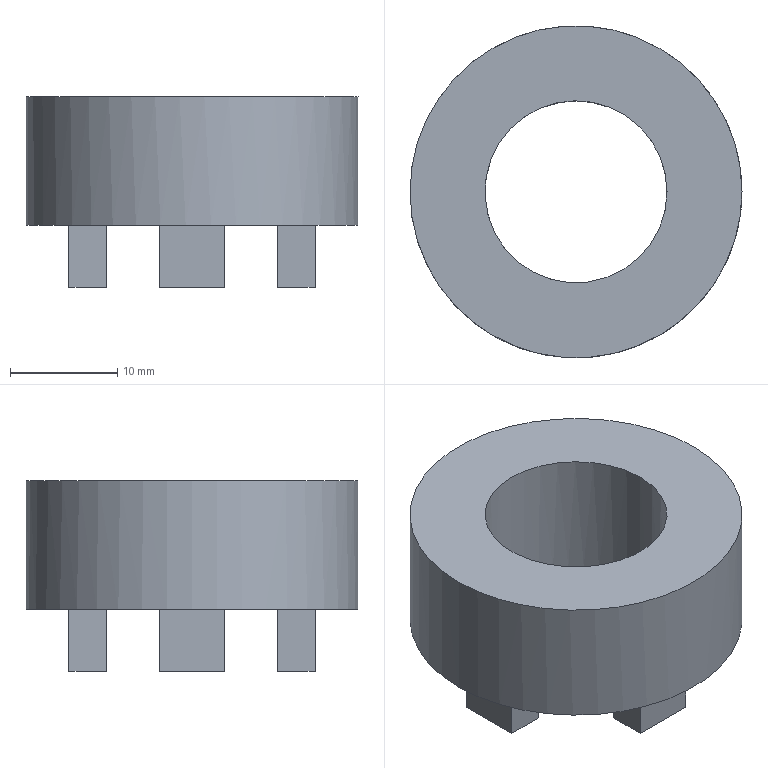Part | NX | features EXTRACT_BODY 3, EXTRUDE 3, DATUM_CSYS 1, LINKED_FACE 1, Pattern Geometry 1, REPLACE_FACE 1, SKETCH 1, UNITE 1 | 1 solid | 20 faces | box 31 x 31 x 17.802 mm | volume 6776 mm3 | plane 18 | cylinder 2 | commonest cylinder face diameters 17 x1 31 x1
STEP:
#1=CARTESIAN_POINT('',(-15.5,0.,-6.));
#2=VERTEX_POINT('',#1);
#3=CARTESIAN_POINT('',(0.,0.,-6.));
#4=DIRECTION('',(0.,0.,1.));
#5=DIRECTION('',(-1.,0.,0.));
#6=AXIS2_PLACEMENT_3D('',#3,#4,#5);
#7=CIRCLE('',#6,15.5);
#8=EDGE_CURVE('',#2,#2,#7,.T.);
#9=ORIENTED_EDGE('',*,*,#8,.F.);
#10=EDGE_LOOP('',(#9));
#11=FACE_BOUND('',#10,.T.);
#12=CARTESIAN_POINT('',(11.5,-3.,-6.));
#13=VERTEX_POINT('',#12);
#14=CARTESIAN_POINT('',(7.953,-3.,-6.));
#15=VERTEX_POINT('',#14);
#16=CARTESIAN_POINT('',(11.5,-3.,-6.));
#17=DIRECTION('',(-1.,0.,0.));
#18=VECTOR('',#17,1000.);
#19=LINE('',#16,#18);
#20=EDGE_CURVE('',#13,#15,#19,.T.);
#21=ORIENTED_EDGE('',*,*,#20,.F.);
#22=CARTESIAN_POINT('',(11.5,3.,-6.));
#23=VERTEX_POINT('',#22);
#24=CARTESIAN_POINT('',(11.5,3.,-6.));
#25=DIRECTION('',(0.,-1.,0.));
#26=VECTOR('',#25,1000.);
#27=LINE('',#24,#26);
#28=EDGE_CURVE('',#23,#13,#27,.T.);
#29=ORIENTED_EDGE('',*,*,#28,.F.);
#30=CARTESIAN_POINT('',(7.953,3.,-6.));
#31=VERTEX_POINT('',#30);
#32=CARTESIAN_POINT('',(7.953,3.,-6.));
#33=DIRECTION('',(1.,0.,0.));
#34=VECTOR('',#33,1000.);
#35=LINE('',#32,#34);
#36=EDGE_CURVE('',#31,#23,#35,.T.);
#37=ORIENTED_EDGE('',*,*,#36,.F.);
#38=CARTESIAN_POINT('',(3.,7.953,-6.));
#39=VERTEX_POINT('',#38);
#40=CARTESIAN_POINT('',(0.,0.,-6.));
#41=DIRECTION('',(0.,0.,1.));
#42=DIRECTION('',(1.,0.,0.));
#43=AXIS2_PLACEMENT_3D('',#40,#41,#42);
#44=CIRCLE('',#43,8.5);
#45=EDGE_CURVE('',#31,#39,#44,.T.);
#46=ORIENTED_EDGE('',*,*,#45,.T.);
#47=CARTESIAN_POINT('',(3.,11.5,-6.));
#48=VERTEX_POINT('',#47);
#49=CARTESIAN_POINT('',(3.,11.5,-6.));
#50=DIRECTION('',(0.,-1.,0.));
#51=VECTOR('',#50,1000.);
#52=LINE('',#49,#51);
#53=EDGE_CURVE('',#48,#39,#52,.T.);
#54=ORIENTED_EDGE('',*,*,#53,.F.);
#55=CARTESIAN_POINT('',(-3.,11.5,-6.));
#56=VERTEX_POINT('',#55);
#57=CARTESIAN_POINT('',(-3.,11.5,-6.));
#58=DIRECTION('',(1.,0.,0.));
#59=VECTOR('',#58,1000.);
#60=LINE('',#57,#59);
#61=EDGE_CURVE('',#56,#48,#60,.T.);
#62=ORIENTED_EDGE('',*,*,#61,.F.);
#63=CARTESIAN_POINT('',(-3.,7.953,-6.));
#64=VERTEX_POINT('',#63);
#65=CARTESIAN_POINT('',(-3.,7.953,-6.));
#66=DIRECTION('',(0.,1.,0.));
#67=VECTOR('',#66,1000.);
#68=LINE('',#65,#67);
#69=EDGE_CURVE('',#64,#56,#68,.T.);
#70=ORIENTED_EDGE('',*,*,#69,.F.);
#71=CARTESIAN_POINT('',(-7.953,3.,-6.));
#72=VERTEX_POINT('',#71);
#73=CARTESIAN_POINT('',(0.,0.,-6.));
#74=DIRECTION('',(0.,0.,1.));
#75=DIRECTION('',(1.,0.,0.));
#76=AXIS2_PLACEMENT_3D('',#73,#74,#75);
#77=CIRCLE('',#76,8.5);
#78=EDGE_CURVE('',#64,#72,#77,.T.);
#79=ORIENTED_EDGE('',*,*,#78,.T.);
#80=CARTESIAN_POINT('',(-11.5,3.,-6.));
#81=VERTEX_POINT('',#80);
#82=CARTESIAN_POINT('',(0.,3.,-6.));
#83=DIRECTION('',(-1.,0.,0.));
#84=VECTOR('',#83,1000.);
#85=LINE('',#82,#84);
#86=EDGE_CURVE('',#72,#81,#85,.T.);
#87=ORIENTED_EDGE('',*,*,#86,.T.);
#88=CARTESIAN_POINT('',(-11.5,-3.,-6.));
#89=VERTEX_POINT('',#88);
#90=CARTESIAN_POINT('',(-11.5,0.,-6.));
#91=DIRECTION('',(0.,-1.,0.));
#92=VECTOR('',#91,1000.);
#93=LINE('',#90,#92);
#94=EDGE_CURVE('',#81,#89,#93,.T.);
#95=ORIENTED_EDGE('',*,*,#94,.T.);
#96=CARTESIAN_POINT('',(-7.953,-3.,-6.));
#97=VERTEX_POINT('',#96);
#98=CARTESIAN_POINT('',(0.,-3.,-6.));
#99=DIRECTION('',(1.,0.,0.));
#100=VECTOR('',#99,1000.);
#101=LINE('',#98,#100);
#102=EDGE_CURVE('',#89,#97,#101,.T.);
#103=ORIENTED_EDGE('',*,*,#102,.T.);
#104=CARTESIAN_POINT('',(-3.,-7.953,-6.));
#105=VERTEX_POINT('',#104);
#106=CARTESIAN_POINT('',(0.,0.,-6.));
#107=DIRECTION('',(0.,0.,1.));
#108=DIRECTION('',(1.,0.,0.));
#109=AXIS2_PLACEMENT_3D('',#106,#107,#108);
#110=CIRCLE('',#109,8.5);
#111=EDGE_CURVE('',#97,#105,#110,.T.);
#112=ORIENTED_EDGE('',*,*,#111,.T.);
#113=CARTESIAN_POINT('',(-3.,-11.5,-6.));
#114=VERTEX_POINT('',#113);
#115=CARTESIAN_POINT('',(-3.,-11.5,-6.));
#116=DIRECTION('',(0.,1.,0.));
#117=VECTOR('',#116,1000.);
#118=LINE('',#115,#117);
#119=EDGE_CURVE('',#114,#105,#118,.T.);
#120=ORIENTED_EDGE('',*,*,#119,.F.);
#121=CARTESIAN_POINT('',(3.,-11.5,-6.));
#122=VERTEX_POINT('',#121);
#123=CARTESIAN_POINT('',(3.,-11.5,-6.));
#124=DIRECTION('',(-1.,0.,0.));
#125=VECTOR('',#124,1000.);
#126=LINE('',#123,#125);
#127=EDGE_CURVE('',#122,#114,#126,.T.);
#128=ORIENTED_EDGE('',*,*,#127,.F.);
#129=CARTESIAN_POINT('',(3.,-7.953,-6.));
#130=VERTEX_POINT('',#129);
#131=CARTESIAN_POINT('',(3.,-7.953,-6.));
#132=DIRECTION('',(0.,-1.,0.));
#133=VECTOR('',#132,1000.);
#134=LINE('',#131,#133);
#135=EDGE_CURVE('',#130,#122,#134,.T.);
#136=ORIENTED_EDGE('',*,*,#135,.F.);
#137=CARTESIAN_POINT('',(0.,0.,-6.));
#138=DIRECTION('',(0.,0.,1.));
#139=DIRECTION('',(1.,0.,0.));
#140=AXIS2_PLACEMENT_3D('',#137,#138,#139);
#141=CIRCLE('',#140,8.5);
#142=EDGE_CURVE('',#130,#15,#141,.T.);
#143=ORIENTED_EDGE('',*,*,#142,.T.);
#144=EDGE_LOOP('',(#21,#29,#37,#46,#54,#62,#70,#79,#87,#95,#103,#112,#120,#128,#136,#143));
#145=FACE_BOUND('',#144,.T.);
#146=CARTESIAN_POINT('',(0.,0.,-6.));
#147=DIRECTION('',(0.,0.,1.));
#148=DIRECTION('',(1.,0.,0.));
#149=AXIS2_PLACEMENT_3D('',#146,#147,#148);
#150=PLANE('',#149);
#151=ADVANCED_FACE('',(#11,#145),#150,.F.);
#152=ORIENTED_EDGE('',*,*,#8,.T.);
#153=EDGE_LOOP('',(#152));
#154=FACE_BOUND('',#153,.T.);
#155=CARTESIAN_POINT('',(15.5,0.,6.));
#156=VERTEX_POINT('',#155);
#157=CARTESIAN_POINT('',(0.,0.,6.));
#158=DIRECTION('',(0.,0.,1.));
#159=DIRECTION('',(1.,0.,0.));
#160=AXIS2_PLACEMENT_3D('',#157,#158,#159);
#161=CIRCLE('',#160,15.5);
#162=EDGE_CURVE('',#156,#156,#161,.T.);
#163=ORIENTED_EDGE('',*,*,#162,.F.);
#164=EDGE_LOOP('',(#163));
#165=FACE_BOUND('',#164,.T.);
#166=CARTESIAN_POINT('',(0.,0.,6.));
#167=DIRECTION('',(0.,0.,-1.));
#168=DIRECTION('',(-1.,0.,0.));
#169=AXIS2_PLACEMENT_3D('',#166,#167,#168);
#170=CYLINDRICAL_SURFACE('',#169,15.5);
#171=ADVANCED_FACE('',(#154,#165),#170,.T.);
#172=CARTESIAN_POINT('',(8.5,0.,6.));
#173=VERTEX_POINT('',#172);
#174=CARTESIAN_POINT('',(0.,0.,6.));
#175=DIRECTION('',(0.,0.,1.));
#176=DIRECTION('',(1.,0.,0.));
#177=AXIS2_PLACEMENT_3D('',#174,#175,#176);
#178=CIRCLE('',#177,8.5);
#179=EDGE_CURVE('',#173,#173,#178,.T.);
#180=ORIENTED_EDGE('',*,*,#179,.F.);
#181=EDGE_LOOP('',(#180));
#182=FACE_BOUND('',#181,.T.);
#183=ORIENTED_EDGE('',*,*,#162,.T.);
#184=EDGE_LOOP('',(#183));
#185=FACE_BOUND('',#184,.T.);
#186=CARTESIAN_POINT('',(0.,0.,6.));
#187=DIRECTION('',(0.,0.,1.));
#188=DIRECTION('',(1.,0.,0.));
#189=AXIS2_PLACEMENT_3D('',#186,#187,#188);
#190=PLANE('',#189);
#191=ADVANCED_FACE('',(#182,#185),#190,.T.);
#192=ORIENTED_EDGE('',*,*,#179,.T.);
#193=EDGE_LOOP('',(#192));
#194=FACE_BOUND('',#193,.T.);
#195=ORIENTED_EDGE('',*,*,#111,.F.);
#196=CARTESIAN_POINT('',(-7.953,-3.,-11.802));
#197=VERTEX_POINT('',#196);
#198=CARTESIAN_POINT('',(-7.953,-3.,-6.));
#199=DIRECTION('',(0.,0.,-1.));
#200=VECTOR('',#199,1000.);
#201=LINE('',#198,#200);
#202=EDGE_CURVE('',#97,#197,#201,.T.);
#203=ORIENTED_EDGE('',*,*,#202,.T.);
#204=CARTESIAN_POINT('',(-7.953,3.,-11.802));
#205=VERTEX_POINT('',#204);
#206=CARTESIAN_POINT('',(0.,0.,-11.802));
#207=DIRECTION('',(0.,0.,1.));
#208=DIRECTION('',(-0.9356,0.3529,0.));
#209=AXIS2_PLACEMENT_3D('',#206,#207,#208);
#210=CIRCLE('',#209,8.5);
#211=EDGE_CURVE('',#205,#197,#210,.T.);
#212=ORIENTED_EDGE('',*,*,#211,.F.);
#213=CARTESIAN_POINT('',(-7.953,3.,-6.));
#214=DIRECTION('',(0.,0.,-1.));
#215=VECTOR('',#214,1000.);
#216=LINE('',#213,#215);
#217=EDGE_CURVE('',#72,#205,#216,.T.);
#218=ORIENTED_EDGE('',*,*,#217,.F.);
#219=ORIENTED_EDGE('',*,*,#78,.F.);
#220=CARTESIAN_POINT('',(-3.,7.953,-11.802));
#221=VERTEX_POINT('',#220);
#222=CARTESIAN_POINT('',(-3.,7.953,-6.));
#223=DIRECTION('',(0.,0.,-1.));
#224=VECTOR('',#223,1000.);
#225=LINE('',#222,#224);
#226=EDGE_CURVE('',#64,#221,#225,.T.);
#227=ORIENTED_EDGE('',*,*,#226,.T.);
#228=CARTESIAN_POINT('',(3.,7.953,-11.802));
#229=VERTEX_POINT('',#228);
#230=CARTESIAN_POINT('',(0.,0.,-11.802));
#231=DIRECTION('',(0.,0.,1.));
#232=DIRECTION('',(0.3529,0.9356,0.));
#233=AXIS2_PLACEMENT_3D('',#230,#231,#232);
#234=CIRCLE('',#233,8.5);
#235=EDGE_CURVE('',#229,#221,#234,.T.);
#236=ORIENTED_EDGE('',*,*,#235,.F.);
#237=CARTESIAN_POINT('',(3.,7.953,-6.));
#238=DIRECTION('',(0.,0.,-1.));
#239=VECTOR('',#238,1000.);
#240=LINE('',#237,#239);
#241=EDGE_CURVE('',#39,#229,#240,.T.);
#242=ORIENTED_EDGE('',*,*,#241,.F.);
#243=ORIENTED_EDGE('',*,*,#45,.F.);
#244=CARTESIAN_POINT('',(7.953,3.,-11.802));
#245=VERTEX_POINT('',#244);
#246=CARTESIAN_POINT('',(7.953,3.,-6.));
#247=DIRECTION('',(0.,0.,-1.));
#248=VECTOR('',#247,1000.);
#249=LINE('',#246,#248);
#250=EDGE_CURVE('',#31,#245,#249,.T.);
#251=ORIENTED_EDGE('',*,*,#250,.T.);
#252=CARTESIAN_POINT('',(7.953,-3.,-11.802));
#253=VERTEX_POINT('',#252);
#254=CARTESIAN_POINT('',(0.,0.,-11.802));
#255=DIRECTION('',(0.,0.,1.));
#256=DIRECTION('',(0.9356,-0.3529,0.));
#257=AXIS2_PLACEMENT_3D('',#254,#255,#256);
#258=CIRCLE('',#257,8.5);
#259=EDGE_CURVE('',#253,#245,#258,.T.);
#260=ORIENTED_EDGE('',*,*,#259,.F.);
#261=CARTESIAN_POINT('',(7.953,-3.,-6.));
#262=DIRECTION('',(0.,0.,-1.));
#263=VECTOR('',#262,1000.);
#264=LINE('',#261,#263);
#265=EDGE_CURVE('',#15,#253,#264,.T.);
#266=ORIENTED_EDGE('',*,*,#265,.F.);
#267=ORIENTED_EDGE('',*,*,#142,.F.);
#268=CARTESIAN_POINT('',(3.,-7.953,-11.802));
#269=VERTEX_POINT('',#268);
#270=CARTESIAN_POINT('',(3.,-7.953,-6.));
#271=DIRECTION('',(0.,0.,-1.));
#272=VECTOR('',#271,1000.);
#273=LINE('',#270,#272);
#274=EDGE_CURVE('',#130,#269,#273,.T.);
#275=ORIENTED_EDGE('',*,*,#274,.T.);
#276=CARTESIAN_POINT('',(-3.,-7.953,-11.802));
#277=VERTEX_POINT('',#276);
#278=CARTESIAN_POINT('',(0.,0.,-11.802));
#279=DIRECTION('',(0.,0.,1.));
#280=DIRECTION('',(-0.3529,-0.9356,0.));
#281=AXIS2_PLACEMENT_3D('',#278,#279,#280);
#282=CIRCLE('',#281,8.5);
#283=EDGE_CURVE('',#277,#269,#282,.T.);
#284=ORIENTED_EDGE('',*,*,#283,.F.);
#285=CARTESIAN_POINT('',(-3.,-7.953,-6.));
#286=DIRECTION('',(0.,0.,-1.));
#287=VECTOR('',#286,1000.);
#288=LINE('',#285,#287);
#289=EDGE_CURVE('',#105,#277,#288,.T.);
#290=ORIENTED_EDGE('',*,*,#289,.F.);
#291=EDGE_LOOP('',(#195,#203,#212,#218,#219,#227,#236,#242,#243,#251,#260,#266,#267,#275,#284,#290));
#292=FACE_BOUND('',#291,.T.);
#293=CARTESIAN_POINT('',(0.,0.,18.198));
#294=DIRECTION('',(0.,0.,-1.));
#295=DIRECTION('',(-1.,0.,0.));
#296=AXIS2_PLACEMENT_3D('',#293,#294,#295);
#297=CYLINDRICAL_SURFACE('',#296,8.5);
#298=ADVANCED_FACE('',(#194,#292),#297,.F.);
#299=CARTESIAN_POINT('',(-3.,-11.5,-11.802));
#300=VERTEX_POINT('',#299);
#301=CARTESIAN_POINT('',(-3.,-11.5,-11.802));
#302=DIRECTION('',(0.,1.,0.));
#303=VECTOR('',#302,1000.);
#304=LINE('',#301,#303);
#305=EDGE_CURVE('',#300,#277,#304,.T.);
#306=ORIENTED_EDGE('',*,*,#305,.F.);
#307=CARTESIAN_POINT('',(-3.,-11.5,-6.));
#308=DIRECTION('',(0.,0.,-1.));
#309=VECTOR('',#308,1000.);
#310=LINE('',#307,#309);
#311=EDGE_CURVE('',#114,#300,#310,.T.);
#312=ORIENTED_EDGE('',*,*,#311,.F.);
#313=ORIENTED_EDGE('',*,*,#119,.T.);
#314=ORIENTED_EDGE('',*,*,#289,.T.);
#315=EDGE_LOOP('',(#306,#312,#313,#314));
#316=FACE_BOUND('',#315,.T.);
#317=CARTESIAN_POINT('',(-3.,-11.5,-6.));
#318=DIRECTION('',(-1.,0.,0.));
#319=DIRECTION('',(0.,0.,1.));
#320=AXIS2_PLACEMENT_3D('',#317,#318,#319);
#321=PLANE('',#320);
#322=ADVANCED_FACE('',(#316),#321,.T.);
#323=CARTESIAN_POINT('',(3.,-11.5,-11.802));
#324=VERTEX_POINT('',#323);
#325=CARTESIAN_POINT('',(3.,-7.953,-11.802));
#326=DIRECTION('',(0.,-1.,0.));
#327=VECTOR('',#326,1000.);
#328=LINE('',#325,#327);
#329=EDGE_CURVE('',#269,#324,#328,.T.);
#330=ORIENTED_EDGE('',*,*,#329,.F.);
#331=ORIENTED_EDGE('',*,*,#274,.F.);
#332=ORIENTED_EDGE('',*,*,#135,.T.);
#333=CARTESIAN_POINT('',(3.,-11.5,-6.));
#334=DIRECTION('',(0.,0.,-1.));
#335=VECTOR('',#334,1000.);
#336=LINE('',#333,#335);
#337=EDGE_CURVE('',#122,#324,#336,.T.);
#338=ORIENTED_EDGE('',*,*,#337,.T.);
#339=EDGE_LOOP('',(#330,#331,#332,#338));
#340=FACE_BOUND('',#339,.T.);
#341=CARTESIAN_POINT('',(3.,-7.953,-6.));
#342=DIRECTION('',(1.,0.,0.));
#343=DIRECTION('',(0.,0.,-1.));
#344=AXIS2_PLACEMENT_3D('',#341,#342,#343);
#345=PLANE('',#344);
#346=ADVANCED_FACE('',(#340),#345,.T.);
#347=CARTESIAN_POINT('',(3.,-11.5,-11.802));
#348=DIRECTION('',(-1.,0.,0.));
#349=VECTOR('',#348,1000.);
#350=LINE('',#347,#349);
#351=EDGE_CURVE('',#324,#300,#350,.T.);
#352=ORIENTED_EDGE('',*,*,#351,.F.);
#353=ORIENTED_EDGE('',*,*,#337,.F.);
#354=ORIENTED_EDGE('',*,*,#127,.T.);
#355=ORIENTED_EDGE('',*,*,#311,.T.);
#356=EDGE_LOOP('',(#352,#353,#354,#355));
#357=FACE_BOUND('',#356,.T.);
#358=CARTESIAN_POINT('',(3.,-11.5,-6.));
#359=DIRECTION('',(0.,-1.,0.));
#360=DIRECTION('',(0.,0.,-1.));
#361=AXIS2_PLACEMENT_3D('',#358,#359,#360);
#362=PLANE('',#361);
#363=ADVANCED_FACE('',(#357),#362,.T.);
#364=ORIENTED_EDGE('',*,*,#305,.T.);
#365=ORIENTED_EDGE('',*,*,#283,.T.);
#366=ORIENTED_EDGE('',*,*,#329,.T.);
#367=ORIENTED_EDGE('',*,*,#351,.T.);
#368=EDGE_LOOP('',(#364,#365,#366,#367));
#369=FACE_BOUND('',#368,.T.);
#370=CARTESIAN_POINT('',(0.,0.,-11.802));
#371=DIRECTION('',(0.,0.,1.));
#372=DIRECTION('',(1.,0.,0.));
#373=AXIS2_PLACEMENT_3D('',#370,#371,#372);
#374=PLANE('',#373);
#375=ADVANCED_FACE('',(#369),#374,.F.);
#376=ORIENTED_EDGE('',*,*,#94,.F.);
#377=CARTESIAN_POINT('',(-11.5,3.,-11.802));
#378=VERTEX_POINT('',#377);
#379=CARTESIAN_POINT('',(-11.5,3.,-6.));
#380=DIRECTION('',(0.,0.,-1.));
#381=VECTOR('',#380,1000.);
#382=LINE('',#379,#381);
#383=EDGE_CURVE('',#81,#378,#382,.T.);
#384=ORIENTED_EDGE('',*,*,#383,.T.);
#385=CARTESIAN_POINT('',(-11.5,-3.,-11.802));
#386=VERTEX_POINT('',#385);
#387=CARTESIAN_POINT('',(-11.5,-3.,-11.802));
#388=DIRECTION('',(0.,1.,0.));
#389=VECTOR('',#388,1000.);
#390=LINE('',#387,#389);
#391=EDGE_CURVE('',#386,#378,#390,.T.);
#392=ORIENTED_EDGE('',*,*,#391,.F.);
#393=CARTESIAN_POINT('',(-11.5,-3.,-6.));
#394=DIRECTION('',(0.,0.,-1.));
#395=VECTOR('',#394,1000.);
#396=LINE('',#393,#395);
#397=EDGE_CURVE('',#89,#386,#396,.T.);
#398=ORIENTED_EDGE('',*,*,#397,.F.);
#399=EDGE_LOOP('',(#376,#384,#392,#398));
#400=FACE_BOUND('',#399,.T.);
#401=CARTESIAN_POINT('',(-11.5,-3.,-6.));
#402=DIRECTION('',(-1.,0.,0.));
#403=DIRECTION('',(0.,0.,-1.));
#404=AXIS2_PLACEMENT_3D('',#401,#402,#403);
#405=PLANE('',#404);
#406=ADVANCED_FACE('',(#400),#405,.T.);
#407=ORIENTED_EDGE('',*,*,#86,.F.);
#408=ORIENTED_EDGE('',*,*,#217,.T.);
#409=CARTESIAN_POINT('',(-11.5,3.,-11.802));
#410=DIRECTION('',(1.,0.,0.));
#411=VECTOR('',#410,1000.);
#412=LINE('',#409,#411);
#413=EDGE_CURVE('',#378,#205,#412,.T.);
#414=ORIENTED_EDGE('',*,*,#413,.F.);
#415=ORIENTED_EDGE('',*,*,#383,.F.);
#416=EDGE_LOOP('',(#407,#408,#414,#415));
#417=FACE_BOUND('',#416,.T.);
#418=CARTESIAN_POINT('',(-11.5,3.,-6.));
#419=DIRECTION('',(0.,1.,0.));
#420=DIRECTION('',(0.,0.,1.));
#421=AXIS2_PLACEMENT_3D('',#418,#419,#420);
#422=PLANE('',#421);
#423=ADVANCED_FACE('',(#417),#422,.T.);
#424=ORIENTED_EDGE('',*,*,#102,.F.);
#425=ORIENTED_EDGE('',*,*,#397,.T.);
#426=CARTESIAN_POINT('',(-7.953,-3.,-11.802));
#427=DIRECTION('',(-1.,0.,0.));
#428=VECTOR('',#427,1000.);
#429=LINE('',#426,#428);
#430=EDGE_CURVE('',#197,#386,#429,.T.);
#431=ORIENTED_EDGE('',*,*,#430,.F.);
#432=ORIENTED_EDGE('',*,*,#202,.F.);
#433=EDGE_LOOP('',(#424,#425,#431,#432));
#434=FACE_BOUND('',#433,.T.);
#435=CARTESIAN_POINT('',(-7.953,-3.,-6.));
#436=DIRECTION('',(0.,-1.,0.));
#437=DIRECTION('',(0.,0.,-1.));
#438=AXIS2_PLACEMENT_3D('',#435,#436,#437);
#439=PLANE('',#438);
#440=ADVANCED_FACE('',(#434),#439,.T.);
#441=ORIENTED_EDGE('',*,*,#413,.T.);
#442=ORIENTED_EDGE('',*,*,#211,.T.);
#443=ORIENTED_EDGE('',*,*,#430,.T.);
#444=ORIENTED_EDGE('',*,*,#391,.T.);
#445=EDGE_LOOP('',(#441,#442,#443,#444));
#446=FACE_BOUND('',#445,.T.);
#447=CARTESIAN_POINT('',(0.,0.,-11.802));
#448=DIRECTION('',(0.,0.,1.));
#449=DIRECTION('',(0.,-1.,0.));
#450=AXIS2_PLACEMENT_3D('',#447,#448,#449);
#451=PLANE('',#450);
#452=ADVANCED_FACE('',(#446),#451,.F.);
#453=CARTESIAN_POINT('',(3.,11.5,-11.802));
#454=VERTEX_POINT('',#453);
#455=CARTESIAN_POINT('',(3.,11.5,-11.802));
#456=DIRECTION('',(0.,-1.,0.));
#457=VECTOR('',#456,1000.);
#458=LINE('',#455,#457);
#459=EDGE_CURVE('',#454,#229,#458,.T.);
#460=ORIENTED_EDGE('',*,*,#459,.F.);
#461=CARTESIAN_POINT('',(3.,11.5,-6.));
#462=DIRECTION('',(0.,0.,-1.));
#463=VECTOR('',#462,1000.);
#464=LINE('',#461,#463);
#465=EDGE_CURVE('',#48,#454,#464,.T.);
#466=ORIENTED_EDGE('',*,*,#465,.F.);
#467=ORIENTED_EDGE('',*,*,#53,.T.);
#468=ORIENTED_EDGE('',*,*,#241,.T.);
#469=EDGE_LOOP('',(#460,#466,#467,#468));
#470=FACE_BOUND('',#469,.T.);
#471=CARTESIAN_POINT('',(3.,11.5,-6.));
#472=DIRECTION('',(1.,0.,0.));
#473=DIRECTION('',(0.,0.,1.));
#474=AXIS2_PLACEMENT_3D('',#471,#472,#473);
#475=PLANE('',#474);
#476=ADVANCED_FACE('',(#470),#475,.T.);
#477=CARTESIAN_POINT('',(-3.,11.5,-11.802));
#478=VERTEX_POINT('',#477);
#479=CARTESIAN_POINT('',(-3.,7.953,-11.802));
#480=DIRECTION('',(0.,1.,0.));
#481=VECTOR('',#480,1000.);
#482=LINE('',#479,#481);
#483=EDGE_CURVE('',#221,#478,#482,.T.);
#484=ORIENTED_EDGE('',*,*,#483,.F.);
#485=ORIENTED_EDGE('',*,*,#226,.F.);
#486=ORIENTED_EDGE('',*,*,#69,.T.);
#487=CARTESIAN_POINT('',(-3.,11.5,-6.));
#488=DIRECTION('',(0.,0.,-1.));
#489=VECTOR('',#488,1000.);
#490=LINE('',#487,#489);
#491=EDGE_CURVE('',#56,#478,#490,.T.);
#492=ORIENTED_EDGE('',*,*,#491,.T.);
#493=EDGE_LOOP('',(#484,#485,#486,#492));
#494=FACE_BOUND('',#493,.T.);
#495=CARTESIAN_POINT('',(-3.,7.953,-6.));
#496=DIRECTION('',(-1.,0.,0.));
#497=DIRECTION('',(0.,0.,-1.));
#498=AXIS2_PLACEMENT_3D('',#495,#496,#497);
#499=PLANE('',#498);
#500=ADVANCED_FACE('',(#494),#499,.T.);
#501=CARTESIAN_POINT('',(-3.,11.5,-11.802));
#502=DIRECTION('',(1.,0.,0.));
#503=VECTOR('',#502,1000.);
#504=LINE('',#501,#503);
#505=EDGE_CURVE('',#478,#454,#504,.T.);
#506=ORIENTED_EDGE('',*,*,#505,.F.);
#507=ORIENTED_EDGE('',*,*,#491,.F.);
#508=ORIENTED_EDGE('',*,*,#61,.T.);
#509=ORIENTED_EDGE('',*,*,#465,.T.);
#510=EDGE_LOOP('',(#506,#507,#508,#509));
#511=FACE_BOUND('',#510,.T.);
#512=CARTESIAN_POINT('',(-3.,11.5,-6.));
#513=DIRECTION('',(0.,1.,0.));
#514=DIRECTION('',(0.,0.,-1.));
#515=AXIS2_PLACEMENT_3D('',#512,#513,#514);
#516=PLANE('',#515);
#517=ADVANCED_FACE('',(#511),#516,.T.);
#518=ORIENTED_EDGE('',*,*,#459,.T.);
#519=ORIENTED_EDGE('',*,*,#235,.T.);
#520=ORIENTED_EDGE('',*,*,#483,.T.);
#521=ORIENTED_EDGE('',*,*,#505,.T.);
#522=EDGE_LOOP('',(#518,#519,#520,#521));
#523=FACE_BOUND('',#522,.T.);
#524=CARTESIAN_POINT('',(0.,0.,-11.802));
#525=DIRECTION('',(0.,0.,1.));
#526=DIRECTION('',(-1.,0.,0.));
#527=AXIS2_PLACEMENT_3D('',#524,#525,#526);
#528=PLANE('',#527);
#529=ADVANCED_FACE('',(#523),#528,.F.);
#530=CARTESIAN_POINT('',(11.5,-3.,-11.802));
#531=VERTEX_POINT('',#530);
#532=CARTESIAN_POINT('',(11.5,-3.,-11.802));
#533=DIRECTION('',(-1.,0.,0.));
#534=VECTOR('',#533,1000.);
#535=LINE('',#532,#534);
#536=EDGE_CURVE('',#531,#253,#535,.T.);
#537=ORIENTED_EDGE('',*,*,#536,.F.);
#538=CARTESIAN_POINT('',(11.5,-3.,-6.));
#539=DIRECTION('',(0.,0.,-1.));
#540=VECTOR('',#539,1000.);
#541=LINE('',#538,#540);
#542=EDGE_CURVE('',#13,#531,#541,.T.);
#543=ORIENTED_EDGE('',*,*,#542,.F.);
#544=ORIENTED_EDGE('',*,*,#20,.T.);
#545=ORIENTED_EDGE('',*,*,#265,.T.);
#546=EDGE_LOOP('',(#537,#543,#544,#545));
#547=FACE_BOUND('',#546,.T.);
#548=CARTESIAN_POINT('',(11.5,-3.,-6.));
#549=DIRECTION('',(0.,-1.,0.));
#550=DIRECTION('',(0.,0.,1.));
#551=AXIS2_PLACEMENT_3D('',#548,#549,#550);
#552=PLANE('',#551);
#553=ADVANCED_FACE('',(#547),#552,.T.);
#554=CARTESIAN_POINT('',(11.5,3.,-11.802));
#555=VERTEX_POINT('',#554);
#556=CARTESIAN_POINT('',(7.953,3.,-11.802));
#557=DIRECTION('',(1.,0.,0.));
#558=VECTOR('',#557,1000.);
#559=LINE('',#556,#558);
#560=EDGE_CURVE('',#245,#555,#559,.T.);
#561=ORIENTED_EDGE('',*,*,#560,.F.);
#562=ORIENTED_EDGE('',*,*,#250,.F.);
#563=ORIENTED_EDGE('',*,*,#36,.T.);
#564=CARTESIAN_POINT('',(11.5,3.,-6.));
#565=DIRECTION('',(0.,0.,-1.));
#566=VECTOR('',#565,1000.);
#567=LINE('',#564,#566);
#568=EDGE_CURVE('',#23,#555,#567,.T.);
#569=ORIENTED_EDGE('',*,*,#568,.T.);
#570=EDGE_LOOP('',(#561,#562,#563,#569));
#571=FACE_BOUND('',#570,.T.);
#572=CARTESIAN_POINT('',(7.953,3.,-6.));
#573=DIRECTION('',(0.,1.,0.));
#574=DIRECTION('',(0.,0.,-1.));
#575=AXIS2_PLACEMENT_3D('',#572,#573,#574);
#576=PLANE('',#575);
#577=ADVANCED_FACE('',(#571),#576,.T.);
#578=CARTESIAN_POINT('',(11.5,3.,-11.802));
#579=DIRECTION('',(0.,-1.,0.));
#580=VECTOR('',#579,1000.);
#581=LINE('',#578,#580);
#582=EDGE_CURVE('',#555,#531,#581,.T.);
#583=ORIENTED_EDGE('',*,*,#582,.F.);
#584=ORIENTED_EDGE('',*,*,#568,.F.);
#585=ORIENTED_EDGE('',*,*,#28,.T.);
#586=ORIENTED_EDGE('',*,*,#542,.T.);
#587=EDGE_LOOP('',(#583,#584,#585,#586));
#588=FACE_BOUND('',#587,.T.);
#589=CARTESIAN_POINT('',(11.5,3.,-6.));
#590=DIRECTION('',(1.,0.,0.));
#591=DIRECTION('',(0.,0.,-1.));
#592=AXIS2_PLACEMENT_3D('',#589,#590,#591);
#593=PLANE('',#592);
#594=ADVANCED_FACE('',(#588),#593,.T.);
#595=ORIENTED_EDGE('',*,*,#536,.T.);
#596=ORIENTED_EDGE('',*,*,#259,.T.);
#597=ORIENTED_EDGE('',*,*,#560,.T.);
#598=ORIENTED_EDGE('',*,*,#582,.T.);
#599=EDGE_LOOP('',(#595,#596,#597,#598));
#600=FACE_BOUND('',#599,.T.);
#601=CARTESIAN_POINT('',(0.,0.,-11.802));
#602=DIRECTION('',(0.,0.,1.));
#603=DIRECTION('',(0.,1.,0.));
#604=AXIS2_PLACEMENT_3D('',#601,#602,#603);
#605=PLANE('',#604);
#606=ADVANCED_FACE('',(#600),#605,.F.);
#607=CLOSED_SHELL('',(#151,#171,#191,#298,#322,#346,#363,#375,#406,#423,#440,#452,#476,#500,#517,#529,#553,#577,#594,#606));
#608=MANIFOLD_SOLID_BREP('',#607);
#609=(LENGTH_UNIT()NAMED_UNIT(*)SI_UNIT(.MILLI.,.METRE.));
#610=UNCERTAINTY_MEASURE_WITH_UNIT(LENGTH_MEASURE(0.00001),#609,'','');
#611=(NAMED_UNIT(*)PLANE_ANGLE_UNIT()SI_UNIT($,.RADIAN.));
#612=(NAMED_UNIT(*)SI_UNIT($,.STERADIAN.)SOLID_ANGLE_UNIT());
#613=(GEOMETRIC_REPRESENTATION_CONTEXT(3)GLOBAL_UNCERTAINTY_ASSIGNED_CONTEXT((#610))GLOBAL_UNIT_ASSIGNED_CONTEXT((#609,#611,#612))REPRESENTATION_CONTEXT('',''));
#614=ADVANCED_BREP_SHAPE_REPRESENTATION('',(#608),#613);